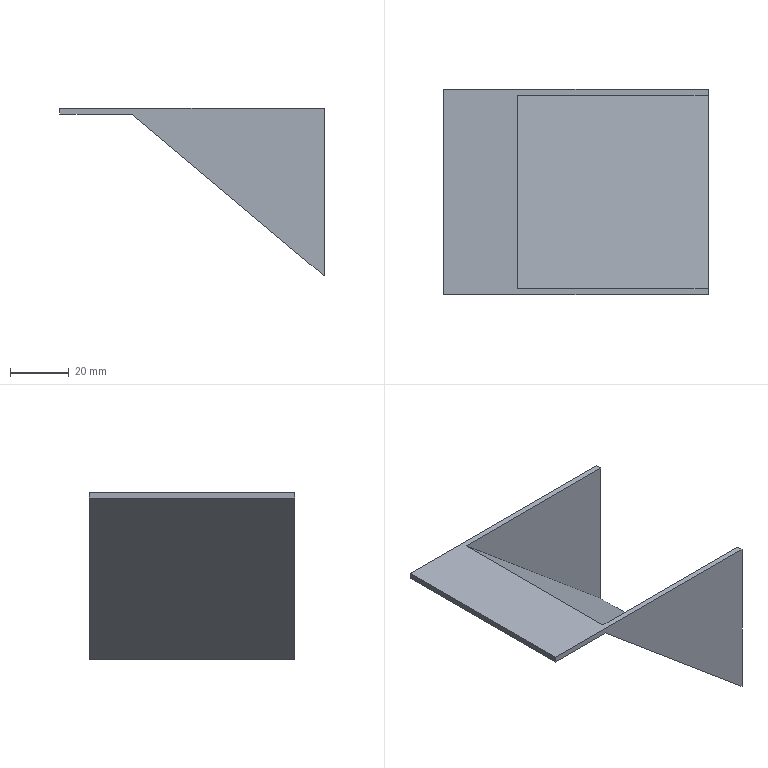Part | NX | features solid 2 | 1 solid | 10 faces | box 90 x 70 x 57.152 mm | volume 22485 mm3 | plane 10
STEP:
#1=CARTESIAN_POINT('',(295.,78.,-175.));
#2=VERTEX_POINT('',#1);
#3=CARTESIAN_POINT('',(360.,78.,-229.541));
#4=VERTEX_POINT('',#3);
#5=CARTESIAN_POINT('',(314.151,78.,-191.07));
#6=DIRECTION('',(0.766,0.,-0.6428));
#7=VECTOR('',#6,1000.);
#8=LINE('',#5,#7);
#9=EDGE_CURVE('',#2,#4,#8,.T.);
#10=ORIENTED_EDGE('',*,*,#9,.F.);
#11=CARTESIAN_POINT('',(295.,12.,-175.));
#12=VERTEX_POINT('',#11);
#13=CARTESIAN_POINT('',(295.,347.701,-175.));
#14=DIRECTION('',(0.,-1.,0.));
#15=VECTOR('',#14,1000.);
#16=LINE('',#13,#15);
#17=EDGE_CURVE('',#12,#2,#16,.F.);
#18=ORIENTED_EDGE('',*,*,#17,.F.);
#19=CARTESIAN_POINT('',(360.,12.,-229.541));
#20=VERTEX_POINT('',#19);
#21=CARTESIAN_POINT('',(314.151,12.,-191.07));
#22=DIRECTION('',(0.766,0.,-0.6428));
#23=VECTOR('',#22,1000.);
#24=LINE('',#21,#23);
#25=EDGE_CURVE('',#20,#12,#24,.F.);
#26=ORIENTED_EDGE('',*,*,#25,.F.);
#27=CARTESIAN_POINT('',(360.,175.,-229.541));
#28=DIRECTION('',(0.,-1.,0.));
#29=VECTOR('',#28,1000.);
#30=LINE('',#27,#29);
#31=EDGE_CURVE('',#20,#4,#30,.F.);
#32=ORIENTED_EDGE('',*,*,#31,.T.);
#33=EDGE_LOOP('',(#10,#18,#26,#32));
#34=FACE_BOUND('',#33,.T.);
#35=CARTESIAN_POINT('',(314.151,-70.,-191.07));
#36=DIRECTION('',(-0.6428,0.,-0.766));
#37=DIRECTION('',(0.766,0.,-0.6428));
#38=AXIS2_PLACEMENT_3D('',#35,#36,#37);
#39=PLANE('',#38);
#40=ADVANCED_FACE('',(#34),#39,.F.);
#41=CARTESIAN_POINT('',(360.,78.,-175.));
#42=VERTEX_POINT('',#41);
#43=CARTESIAN_POINT('',(360.,78.,-191.07));
#44=DIRECTION('',(0.,0.,1.));
#45=VECTOR('',#44,1000.);
#46=LINE('',#43,#45);
#47=EDGE_CURVE('',#42,#4,#46,.F.);
#48=ORIENTED_EDGE('',*,*,#47,.T.);
#49=ORIENTED_EDGE('',*,*,#31,.F.);
#50=CARTESIAN_POINT('',(360.,12.,-175.));
#51=VERTEX_POINT('',#50);
#52=CARTESIAN_POINT('',(360.,12.,0.));
#53=DIRECTION('',(0.,0.,-1.));
#54=VECTOR('',#53,1000.);
#55=LINE('',#52,#54);
#56=EDGE_CURVE('',#51,#20,#55,.T.);
#57=ORIENTED_EDGE('',*,*,#56,.F.);
#58=CARTESIAN_POINT('',(360.,10.,-175.));
#59=VERTEX_POINT('',#58);
#60=CARTESIAN_POINT('',(360.,10.,-175.));
#61=DIRECTION('',(0.,-1.,0.));
#62=VECTOR('',#61,1000.);
#63=LINE('',#60,#62);
#64=EDGE_CURVE('',#51,#59,#63,.T.);
#65=ORIENTED_EDGE('',*,*,#64,.T.);
#66=CARTESIAN_POINT('',(360.,10.,-232.152));
#67=VERTEX_POINT('',#66);
#68=CARTESIAN_POINT('',(360.,10.,0.));
#69=DIRECTION('',(0.,0.,-1.));
#70=VECTOR('',#69,1000.);
#71=LINE('',#68,#70);
#72=EDGE_CURVE('',#59,#67,#71,.T.);
#73=ORIENTED_EDGE('',*,*,#72,.T.);
#74=CARTESIAN_POINT('',(360.,80.,-232.152));
#75=VERTEX_POINT('',#74);
#76=CARTESIAN_POINT('',(360.,175.,-232.152));
#77=DIRECTION('',(0.,-1.,0.));
#78=VECTOR('',#77,1000.);
#79=LINE('',#76,#78);
#80=EDGE_CURVE('',#67,#75,#79,.F.);
#81=ORIENTED_EDGE('',*,*,#80,.T.);
#82=CARTESIAN_POINT('',(360.,80.,-175.));
#83=VERTEX_POINT('',#82);
#84=CARTESIAN_POINT('',(360.,80.,-191.07));
#85=DIRECTION('',(0.,0.,1.));
#86=VECTOR('',#85,1000.);
#87=LINE('',#84,#86);
#88=EDGE_CURVE('',#83,#75,#87,.F.);
#89=ORIENTED_EDGE('',*,*,#88,.F.);
#90=CARTESIAN_POINT('',(360.,80.,-175.));
#91=DIRECTION('',(0.,1.,0.));
#92=VECTOR('',#91,1000.);
#93=LINE('',#90,#92);
#94=EDGE_CURVE('',#83,#42,#93,.F.);
#95=ORIENTED_EDGE('',*,*,#94,.T.);
#96=EDGE_LOOP('',(#48,#49,#57,#65,#73,#81,#89,#95));
#97=FACE_BOUND('',#96,.T.);
#98=CARTESIAN_POINT('',(360.,175.,0.));
#99=DIRECTION('',(-1.,0.,0.));
#100=DIRECTION('',(0.,0.,1.));
#101=AXIS2_PLACEMENT_3D('',#98,#99,#100);
#102=PLANE('',#101);
#103=ADVANCED_FACE('',(#97),#102,.F.);
#104=CARTESIAN_POINT('',(294.272,80.,-177.));
#105=VERTEX_POINT('',#104);
#106=CARTESIAN_POINT('',(270.,80.,-177.));
#107=VERTEX_POINT('',#106);
#108=CARTESIAN_POINT('',(314.151,80.,-177.));
#109=DIRECTION('',(-1.,0.,0.));
#110=VECTOR('',#109,1000.);
#111=LINE('',#108,#110);
#112=EDGE_CURVE('',#105,#107,#111,.T.);
#113=ORIENTED_EDGE('',*,*,#112,.T.);
#114=CARTESIAN_POINT('',(270.,80.,-175.));
#115=VERTEX_POINT('',#114);
#116=CARTESIAN_POINT('',(270.,80.,-191.07));
#117=DIRECTION('',(0.,0.,1.));
#118=VECTOR('',#117,1000.);
#119=LINE('',#116,#118);
#120=EDGE_CURVE('',#107,#115,#119,.T.);
#121=ORIENTED_EDGE('',*,*,#120,.T.);
#122=CARTESIAN_POINT('',(295.,80.,-175.));
#123=DIRECTION('',(1.,0.,0.));
#124=VECTOR('',#123,1000.);
#125=LINE('',#122,#124);
#126=EDGE_CURVE('',#83,#115,#125,.F.);
#127=ORIENTED_EDGE('',*,*,#126,.F.);
#128=ORIENTED_EDGE('',*,*,#88,.T.);
#129=CARTESIAN_POINT('',(312.866,80.,-192.602));
#130=DIRECTION('',(-0.766,0.,0.6428));
#131=VECTOR('',#130,1000.);
#132=LINE('',#129,#131);
#133=EDGE_CURVE('',#75,#105,#132,.T.);
#134=ORIENTED_EDGE('',*,*,#133,.T.);
#135=EDGE_LOOP('',(#113,#121,#127,#128,#134));
#136=FACE_BOUND('',#135,.T.);
#137=CARTESIAN_POINT('',(314.151,80.,-191.07));
#138=DIRECTION('',(0.,1.,0.));
#139=DIRECTION('',(-0.766,0.,0.6428));
#140=AXIS2_PLACEMENT_3D('',#137,#138,#139);
#141=PLANE('',#140);
#142=ADVANCED_FACE('',(#136),#141,.T.);
#143=CARTESIAN_POINT('',(294.272,10.,-177.));
#144=VERTEX_POINT('',#143);
#145=CARTESIAN_POINT('',(312.866,10.,-192.602));
#146=DIRECTION('',(0.766,0.,-0.6428));
#147=VECTOR('',#146,1000.);
#148=LINE('',#145,#147);
#149=EDGE_CURVE('',#67,#144,#148,.F.);
#150=ORIENTED_EDGE('',*,*,#149,.F.);
#151=ORIENTED_EDGE('',*,*,#72,.F.);
#152=CARTESIAN_POINT('',(270.,10.,-175.));
#153=VERTEX_POINT('',#152);
#154=CARTESIAN_POINT('',(314.151,10.,-175.));
#155=DIRECTION('',(-1.,0.,0.));
#156=VECTOR('',#155,1000.);
#157=LINE('',#154,#156);
#158=EDGE_CURVE('',#59,#153,#157,.T.);
#159=ORIENTED_EDGE('',*,*,#158,.T.);
#160=CARTESIAN_POINT('',(270.,10.,-177.));
#161=VERTEX_POINT('',#160);
#162=CARTESIAN_POINT('',(270.,10.,0.));
#163=DIRECTION('',(0.,0.,-1.));
#164=VECTOR('',#163,1000.);
#165=LINE('',#162,#164);
#166=EDGE_CURVE('',#161,#153,#165,.F.);
#167=ORIENTED_EDGE('',*,*,#166,.F.);
#168=CARTESIAN_POINT('',(295.,10.,-177.));
#169=DIRECTION('',(1.,0.,0.));
#170=VECTOR('',#169,1000.);
#171=LINE('',#168,#170);
#172=EDGE_CURVE('',#144,#161,#171,.F.);
#173=ORIENTED_EDGE('',*,*,#172,.F.);
#174=EDGE_LOOP('',(#150,#151,#159,#167,#173));
#175=FACE_BOUND('',#174,.T.);
#176=CARTESIAN_POINT('',(314.151,10.,-191.07));
#177=DIRECTION('',(0.,1.,0.));
#178=DIRECTION('',(-0.766,0.,0.6428));
#179=AXIS2_PLACEMENT_3D('',#176,#177,#178);
#180=PLANE('',#179);
#181=ADVANCED_FACE('',(#175),#180,.F.);
#182=ORIENTED_EDGE('',*,*,#133,.F.);
#183=ORIENTED_EDGE('',*,*,#80,.F.);
#184=ORIENTED_EDGE('',*,*,#149,.T.);
#185=CARTESIAN_POINT('',(294.272,-70.,-177.));
#186=DIRECTION('',(0.,1.,0.));
#187=VECTOR('',#186,1000.);
#188=LINE('',#185,#187);
#189=EDGE_CURVE('',#144,#105,#188,.T.);
#190=ORIENTED_EDGE('',*,*,#189,.T.);
#191=EDGE_LOOP('',(#182,#183,#184,#190));
#192=FACE_BOUND('',#191,.T.);
#193=CARTESIAN_POINT('',(312.866,-70.,-192.602));
#194=DIRECTION('',(-0.6428,0.,-0.766));
#195=DIRECTION('',(0.766,0.,-0.6428));
#196=AXIS2_PLACEMENT_3D('',#193,#194,#195);
#197=PLANE('',#196);
#198=ADVANCED_FACE('',(#192),#197,.T.);
#199=ORIENTED_EDGE('',*,*,#112,.F.);
#200=ORIENTED_EDGE('',*,*,#189,.F.);
#201=ORIENTED_EDGE('',*,*,#172,.T.);
#202=CARTESIAN_POINT('',(270.,-70.,-177.));
#203=DIRECTION('',(0.,1.,0.));
#204=VECTOR('',#203,1000.);
#205=LINE('',#202,#204);
#206=EDGE_CURVE('',#161,#107,#205,.T.);
#207=ORIENTED_EDGE('',*,*,#206,.T.);
#208=EDGE_LOOP('',(#199,#200,#201,#207));
#209=FACE_BOUND('',#208,.T.);
#210=CARTESIAN_POINT('',(295.,-70.,-177.));
#211=DIRECTION('',(0.,0.,-1.));
#212=DIRECTION('',(0.,1.,0.));
#213=AXIS2_PLACEMENT_3D('',#210,#211,#212);
#214=PLANE('',#213);
#215=ADVANCED_FACE('',(#209),#214,.T.);
#216=ORIENTED_EDGE('',*,*,#126,.T.);
#217=CARTESIAN_POINT('',(270.,70.,-175.));
#218=DIRECTION('',(0.,-1.,0.));
#219=VECTOR('',#218,1000.);
#220=LINE('',#217,#219);
#221=EDGE_CURVE('',#153,#115,#220,.F.);
#222=ORIENTED_EDGE('',*,*,#221,.F.);
#223=ORIENTED_EDGE('',*,*,#158,.F.);
#224=ORIENTED_EDGE('',*,*,#64,.F.);
#225=CARTESIAN_POINT('',(314.151,12.,-175.));
#226=DIRECTION('',(-1.,0.,0.));
#227=VECTOR('',#226,1000.);
#228=LINE('',#225,#227);
#229=EDGE_CURVE('',#51,#12,#228,.T.);
#230=ORIENTED_EDGE('',*,*,#229,.T.);
#231=ORIENTED_EDGE('',*,*,#17,.T.);
#232=CARTESIAN_POINT('',(295.,78.,-175.));
#233=DIRECTION('',(1.,0.,0.));
#234=VECTOR('',#233,1000.);
#235=LINE('',#232,#234);
#236=EDGE_CURVE('',#42,#2,#235,.F.);
#237=ORIENTED_EDGE('',*,*,#236,.F.);
#238=ORIENTED_EDGE('',*,*,#94,.F.);
#239=EDGE_LOOP('',(#216,#222,#223,#224,#230,#231,#237,#238));
#240=FACE_BOUND('',#239,.T.);
#241=CARTESIAN_POINT('',(295.,-70.,-175.));
#242=DIRECTION('',(0.,0.,-1.));
#243=DIRECTION('',(0.,1.,0.));
#244=AXIS2_PLACEMENT_3D('',#241,#242,#243);
#245=PLANE('',#244);
#246=ADVANCED_FACE('',(#240),#245,.F.);
#247=ORIENTED_EDGE('',*,*,#120,.F.);
#248=ORIENTED_EDGE('',*,*,#206,.F.);
#249=ORIENTED_EDGE('',*,*,#166,.T.);
#250=ORIENTED_EDGE('',*,*,#221,.T.);
#251=EDGE_LOOP('',(#247,#248,#249,#250));
#252=FACE_BOUND('',#251,.T.);
#253=CARTESIAN_POINT('',(270.,70.,0.));
#254=DIRECTION('',(-1.,0.,0.));
#255=DIRECTION('',(0.,0.,-1.));
#256=AXIS2_PLACEMENT_3D('',#253,#254,#255);
#257=PLANE('',#256);
#258=ADVANCED_FACE('',(#252),#257,.T.);
#259=ORIENTED_EDGE('',*,*,#56,.T.);
#260=ORIENTED_EDGE('',*,*,#25,.T.);
#261=ORIENTED_EDGE('',*,*,#229,.F.);
#262=EDGE_LOOP('',(#259,#260,#261));
#263=FACE_BOUND('',#262,.T.);
#264=CARTESIAN_POINT('',(314.151,12.,-191.07));
#265=DIRECTION('',(0.,1.,0.));
#266=DIRECTION('',(-0.766,0.,0.6428));
#267=AXIS2_PLACEMENT_3D('',#264,#265,#266);
#268=PLANE('',#267);
#269=ADVANCED_FACE('',(#263),#268,.T.);
#270=ORIENTED_EDGE('',*,*,#236,.T.);
#271=ORIENTED_EDGE('',*,*,#9,.T.);
#272=ORIENTED_EDGE('',*,*,#47,.F.);
#273=EDGE_LOOP('',(#270,#271,#272));
#274=FACE_BOUND('',#273,.T.);
#275=CARTESIAN_POINT('',(314.151,78.,-191.07));
#276=DIRECTION('',(0.,1.,0.));
#277=DIRECTION('',(-0.766,0.,0.6428));
#278=AXIS2_PLACEMENT_3D('',#275,#276,#277);
#279=PLANE('',#278);
#280=ADVANCED_FACE('',(#274),#279,.F.);
#281=CLOSED_SHELL('',(#40,#103,#142,#181,#198,#215,#246,#258,#269,#280));
#282=MANIFOLD_SOLID_BREP('',#281);
#283=(LENGTH_UNIT()NAMED_UNIT(*)SI_UNIT(.MILLI.,.METRE.));
#284=UNCERTAINTY_MEASURE_WITH_UNIT(LENGTH_MEASURE(0.00001),#283,'','');
#285=(NAMED_UNIT(*)PLANE_ANGLE_UNIT()SI_UNIT($,.RADIAN.));
#286=(NAMED_UNIT(*)SI_UNIT($,.STERADIAN.)SOLID_ANGLE_UNIT());
#287=(GEOMETRIC_REPRESENTATION_CONTEXT(3)GLOBAL_UNCERTAINTY_ASSIGNED_CONTEXT((#284))GLOBAL_UNIT_ASSIGNED_CONTEXT((#283,#285,#286))REPRESENTATION_CONTEXT('',''));
#288=ADVANCED_BREP_SHAPE_REPRESENTATION('',(#282),#287);